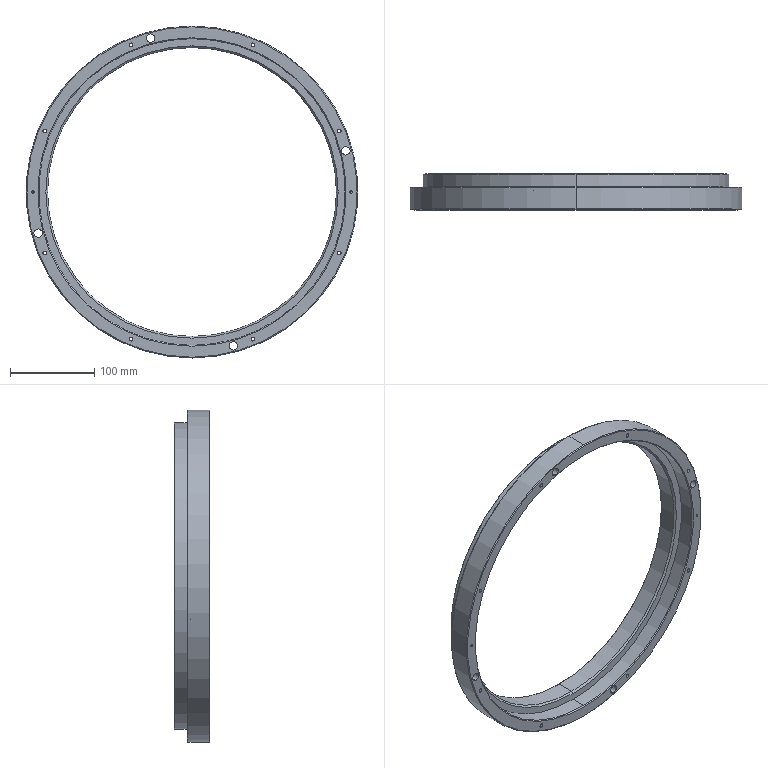Part | NX | features BREP 1 | 1 solid | 146 faces | box 393 x 42.5 x 393 mm | volume 727739 mm3 | cylinder 80 | cone 50 | plane 16 | commonest cylinder face diameters 10 x24 2.5 x16 4.5 x16 3 x8 12.2 x8 363 x4